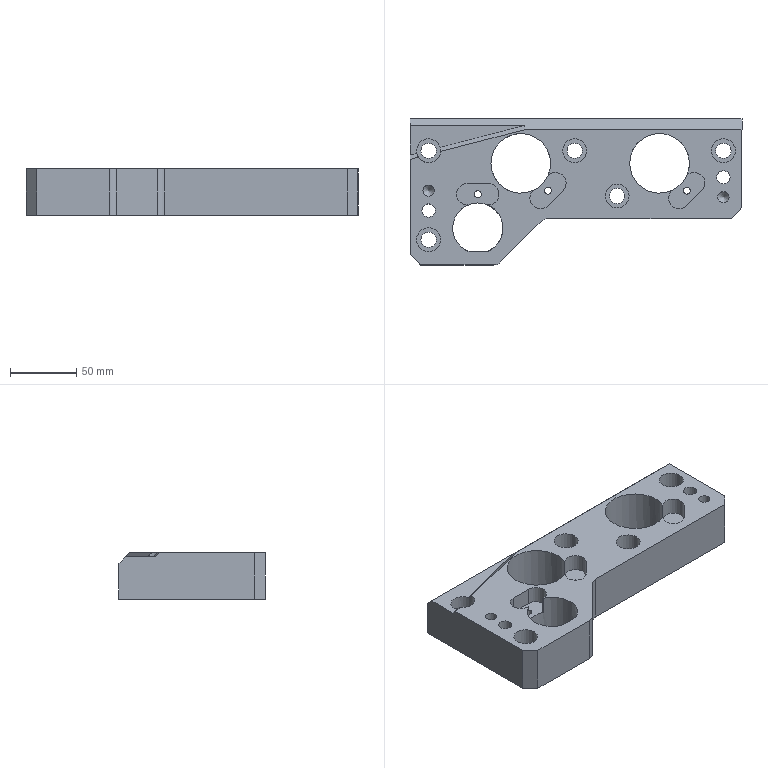Part | STEP file | lll_id4562_x_t | 1 solid | 58 faces | box 250 x 110 x 35 mm | volume 539795 mm3 | plane 28 | cylinder 28 | cone 2 | commonest cylinder face diameters 16 x8 11.509 x5 18.008 x5 5.206 x3 8.506 x2 10 x2